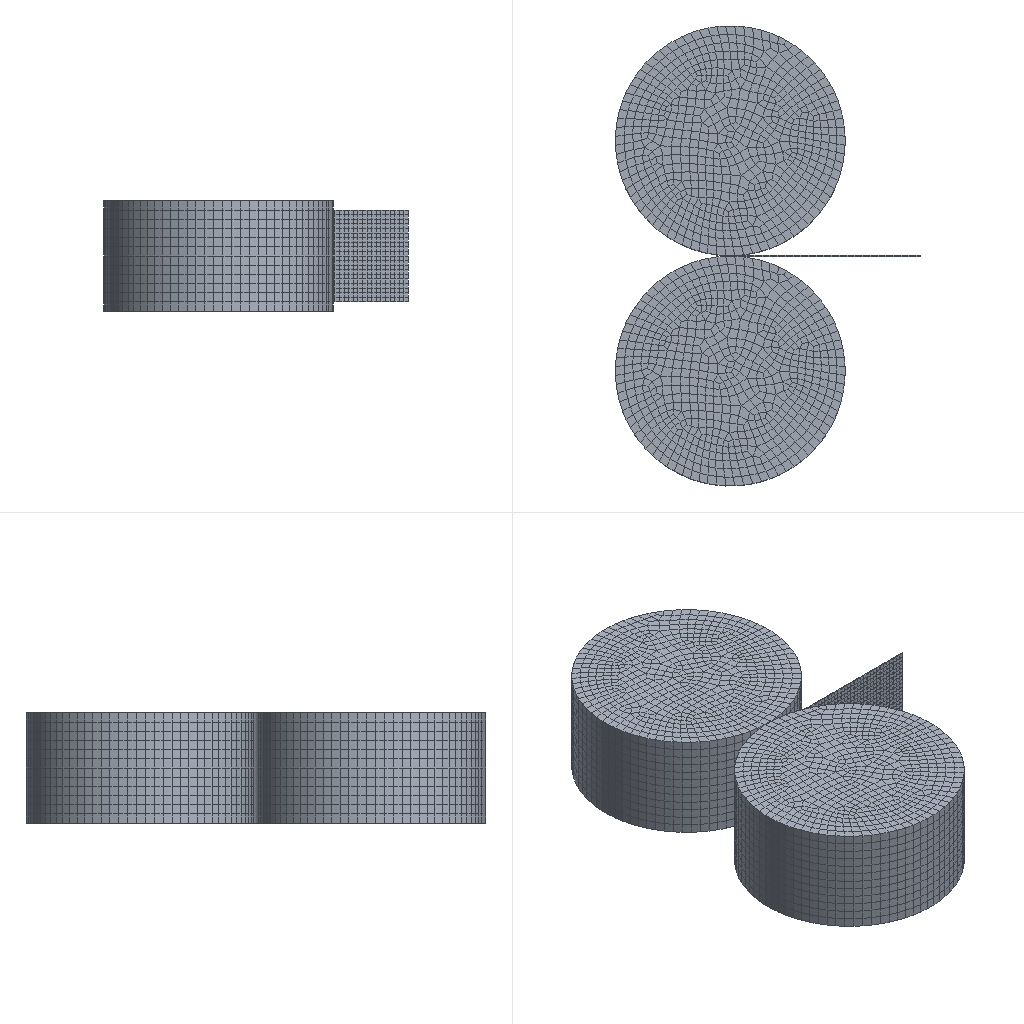Simulation study | abaqus
Set-up summary:
category,name,step,type,value,unit,region
solver,abaqus
solver,version,,,Abaqus/Explicit 2020
units,not stated in the deck,,not stated
analysis,deck,,dynamic temperature-displacement,dynamic temperature-displacement
load_step,Step-1,Step-1,dynamic temperature-displacement
load_step,requested,,,1
mesh,nodes,,,20988
mesh,elements,,,17600
element_type,C3D8RT,,solid,17600
load,load commands in deck,,count,6
bc,support commands in deck,,count,13
material,MATERIAL-1,,in results
material,RIG,,in results
check,setup vs results,,match,"per instance, exact: element labels, types and connectivity; labels of the nodes the elements use; coordinates of those nodes at SINGLE_PRECISION in 3 of 3 instance(s)"
Abaqus input file, long lists of numbers shortened:
*Heading
** Job name: Job-2 Model name: Model-1
** Generated by: Abaqus/CAE 2020
*Preprint, echo=NO, model=NO, history=NO, contact=NO
**
** PARTS
**
*Part, name=rig
*Node
      1,   77.43,  -98.131,           0.
      2,   98.199,  -77.344,           0.
** (9631 more lines like these left out)
*Element, type=C3D8RT
   1,  868,  820,  769,  905,  127,   79,   28,  164
   2,  866,  818,  768, 1365,  125,   77,   27,  624
** (8398 more lines like these left out)
*Nset, nset=Set-1, generate
    1,  9633,     1
*Elset, elset=Set-1, generate
    1,  8400,     1
** Section: rig
*Solid Section, elset=Set-1, material=rig
,
*End Part
**
*Part, name=work
*Node
      1,           0.,        -100.,           1.
      2,           0.,         -95.,           1.
** (1720 more lines like these left out)
*Element, type=C3D8RT
  1,   43,   44,   65,   64,    1,    2,   23,   22
  2,   44,   45,   66,   65,    2,    3,   24,   23
** (798 more lines like these left out)
*Nset, nset=Set-1, generate
    1,  1722,     1
*Elset, elset=Set-1, generate
   1,  800,    1
** Section: Section-1
*Solid Section, elset=Set-1, material=Material-1
,
*End Part
**
**
** ASSEMBLY
**
*Assembly, name=Assembly
**
*Instance, name=rig-1, part=rig
          0.,         125.,        -110.
*End Instance
**
*Instance, name=work-1, part=work
          7.,          0.2,           0.
          7.,          0.2,           0., 8.,          0.2,           0., 90.
*End Instance
**
*Instance, name=rig-1-lin-2-1, part=rig
          0.,       -125.6,        -110.
*End Instance
**
*Node
      1,           0.,         125.,          10.
*Node
      2,           0.,  -125.6,          10.
*Nset, nset=Set-5
 1, 2
*Nset, nset=Set-6, instance=work-1, generate
 1681,  1722,     1
*Elset, elset=Set-6, instance=work-1, generate
 781,  800,    1
*Nset, nset=Set-7, instance=work-1, generate
  1,  42,   1
*Elset, elset=Set-7, instance=work-1, generate
  1,  20,   1
*Nset, nset=Set-8, instance=work-1, generate
 1681,  1722,     1
*Elset, elset=Set-8, instance=work-1, generate
 781,  800,    1
*Nset, nset=Set-9, instance=work-1, generate
    1,  1722,     1
*Elset, elset=Set-9, instance=work-1, generate
   1,  800,    1
*Nset, nset=Set-10
 1,
*Nset, nset=Set-11
 2,
*Nset, nset=Set-12, instance=work-1, generate
    1,  1722,     1
*Elset, elset=Set-12, instance=work-1, generate
   1,  800,    1
*Nset, nset=Set-13, instance=work-1
    1,   21,   22,   42,   43,   63,   64,   84,   85,  105,  106,  126,  127,  147,  148,  168
  169,  189,  190,  210,  211,  231,  232,  252,  253,  273,  274,  294,  295,  315,  316,  336
** (9 more lines like these left out)
*Elset, elset=Set-13, instance=work-1
   1,  20,  21,  40,  41,  60,  61,  80,  81, 100, 101, 120, 121, 140, 141, 160
 161, 180, 181, 200, 201, 220, 221, 240, 241, 260, 261, 280, 281, 300, 301, 320
** (3 more lines like these left out)
*Nset, nset=b_Set-1, instance=rig-1, generate
    1,  9633,     1
*Elset, elset=b_Set-1, instance=rig-1, generate
    1,  8400,     1
*Nset, nset=b_Set-3, instance=rig-1-lin-2-1, generate
    1,  9633,     1
*Elset, elset=b_Set-3, instance=rig-1-lin-2-1, generate
    1,  8400,     1
*Nset, nset=_PickedSet11, internal
 1,
*Nset, nset=_PickedSet13, internal
 2,
*Elset, elset=_Surf-5_S1, internal, instance=work-1, generate
 781,  800,    1
*Elset, elset=_Surf-5_S6, internal, instance=work-1, generate
   1,  781,   20
*Elset, elset=_Surf-5_S2, internal, instance=work-1, generate
  1,  20,   1
*Elset, elset=_Surf-5_S4, internal, instance=work-1, generate
  20,  800,   20
*Elset, elset=_Surf-5_S3, internal, instance=work-1, generate
   1,  800,    1
*Elset, elset=_Surf-5_S5, internal, instance=work-1, generate
   1,  800,    1
*Surface, type=ELEMENT, name=Surf-5
_Surf-5_S1, S1
_Surf-5_S6, S6
_Surf-5_S2, S2
_Surf-5_S4, S4
_Surf-5_S3, S3
_Surf-5_S5, S5
*Elset, elset=_Surf-6_S1, internal, instance=work-1, generate
 781,  800,    1
*Elset, elset=_Surf-6_S2, internal, instance=work-1, generate
  1,  20,   1
*Surface, type=ELEMENT, name=Surf-6
_Surf-6_S1, S1
_Surf-6_S2, S2
*Elset, elset=_Surf-7_S6, internal, instance=work-1, generate
   1,  781,   20
*Elset, elset=_Surf-7_S4, internal, instance=work-1, generate
  20,  800,   20
*Surface, type=ELEMENT, name=Surf-7
_Surf-7_S6, S6
_Surf-7_S4, S4
*Elset, elset=_m_Surf-1_S4, internal, instance=rig-1
    1,    2,    4,    5,    8,   14,   16,   21,   24,   28,   29,   32,   33,   35,   36,   37
   38,   41,   42,   43,   49,   54,   59,   63,   69,   70,   71,   72,   73,   74,   75,   77
** (31 more lines like these left out)
*Elset, elset=_m_Surf-1_S6, internal, instance=rig-1
    3,    6,    7,    9,   10,   11,   12,   13,   17,   18,   20,   22,   30,   34,   39,   46
   48,   50,   52,   55,   56,   57,   60,   61,   62,   65,   66,   67,   68,   76,   90,   96
** (25 more lines like these left out)
*Surface, type=ELEMENT, name=m_Surf-1
_m_Surf-1_S4, S4
_m_Surf-1_S6, S6
*Elset, elset=_m_Surf-3_S4, internal, instance=rig-1-lin-2-1
    1,    2,    4,    5,    8,   14,   16,   21,   24,   28,   29,   32,   33,   35,   36,   37
   38,   41,   42,   43,   49,   54,   59,   63,   69,   70,   71,   72,   73,   74,   75,   77
** (31 more lines like these left out)
*Elset, elset=_m_Surf-3_S6, internal, instance=rig-1-lin-2-1
    3,    6,    7,    9,   10,   11,   12,   13,   17,   18,   20,   22,   30,   34,   39,   46
   48,   50,   52,   55,   56,   57,   60,   61,   62,   65,   66,   67,   68,   76,   90,   96
** (25 more lines like these left out)
*Surface, type=ELEMENT, name=m_Surf-3
_m_Surf-3_S4, S4
_m_Surf-3_S6, S6
*Elset, elset=_s_Surf-1_S5, internal, instance=work-1, generate
   1,  800,    1
*Surface, type=ELEMENT, name=s_Surf-1
_s_Surf-1_S5, S5
*Elset, elset=_s_Surf-3_S3, internal, instance=work-1, generate
   1,  800,    1
*Surface, type=ELEMENT, name=s_Surf-3
_s_Surf-3_S3, S3
** Constraint: Constraint-1
*Rigid Body, ref node=_PickedSet11, elset=b_Set-1
** Constraint: Constraint-2
*Rigid Body, ref node=_PickedSet13, elset=b_Set-3
*End Assembly
*Amplitude, name=Amp-1
             0.,              0.,            0.01,              1.
**
** MATERIALS
**
*Material, name=Material-1
*Conductivity
155.,
*Density
 2.5e-09,
*Elastic
45000., 0.308
*Expansion
 2e-05,
*Plastic
 33.,    0.
 60., 0.017
 85., 0.026
105., 0.034
121., 0.043
136., 0.052
150.,  0.06
165.,  0.07
200., 0.094
230.,  0.12
240., 0.142
*Specific Heat
 9e+08,
*Material, name=rig
*Conductivity
45.,
*Density
 7.8e-09,
*Elastic
210000., 0.3
*Specific Heat
 4.6e+08,
**
** INTERACTION PROPERTIES
**
*Surface Interaction, name=IntProp-1
*Friction
 0.25,
*Surface Behavior, pressure-overclosure=HARD
*Gap Conductance
11.,   0.
 0., 0.01
**
** PREDEFINED FIELDS
**
** Name: Predefined Field-1   Type: Velocity
*Initial Conditions, type=VELOCITY
Set-12, 1, -2000.
Set-12, 2, 0.
Set-12, 3, 0.
** ----------------------------------------------------------------
**
** STEP: Step-1
**
*Step, name=Step-1, nlgeom=YES
*Dynamic Temperature-displacement, Explicit
, 0.02
*Bulk Viscosity
0.06, 1.2
**
** BOUNDARY CONDITIONS
**
** Name: BC-3 Type: 速度/角速度
*Boundary, type=VELOCITY
Set-10, 1, 1
Set-10, 2, 2
Set-10, 3, 3
Set-10, 4, 4
Set-10, 5, 5
Set-10, 6, 6, -120.
** Name: BC-3-Copy Type: 速度/角速度
*Boundary, type=VELOCITY
Set-11, 1, 1
Set-11, 2, 2
Set-11, 3, 3
Set-11, 4, 4
Set-11, 5, 5
Set-11, 6, 6, 120.
**
** LOADS
**
** Name: Load-1   Type: Pressure
*Dsload
Surf-6, P, -20.
** Name: Load-2   Type: Pressure
*Dsload
Surf-7, P, -5.
**
** INTERACTIONS
**
** Interaction: Int-1
*Contact Pair, interaction=IntProp-1, mechanical constraint=KINEMATIC, cpset=Int-1
m_Surf-1, s_Surf-1
** Interaction: Int-1-Copy
*Contact Pair, interaction=IntProp-1, mechanical constraint=KINEMATIC, cpset=Int-1-Copy
m_Surf-3, s_Surf-3
** Interaction: Int-3
*Sfilm
Surf-5, F, 25., 0.016
**
** OUTPUT REQUESTS
**
*Restart, write, number interval=1, time marks=NO
**
** FIELD OUTPUT: F-Output-1
**
*Output, field, number interval=50
*Node Output
A, CF, NT, RF, RFL, RM, RT, U
V
*Element Output, directions=YES
E, EVF, HFL, LE, MISES, MISESMAX, PE, PEEQ, PEEQVAVG, PEVAVG, S, SF, SVAVG, TEMP, YIELDPOT
*Contact Output
CDISP, CSTRESS
**
** HISTORY OUTPUT: H-Output-1
**
*Output, history, variable=PRESELECT
*End Step
Results summary:
result,step,Step-1,completed,increments=137039 time=0.02/0.02
result,analysis,,,"dynamic temperature-displacement, explict"
result,last_loadstep,,,1
result,primary field,,,"U, NT11"
result,reaction total,,FX,0.003054,model units
result,reaction total,,FY,-0.005717,model units
result,reaction total,,FZ,0.0,model units